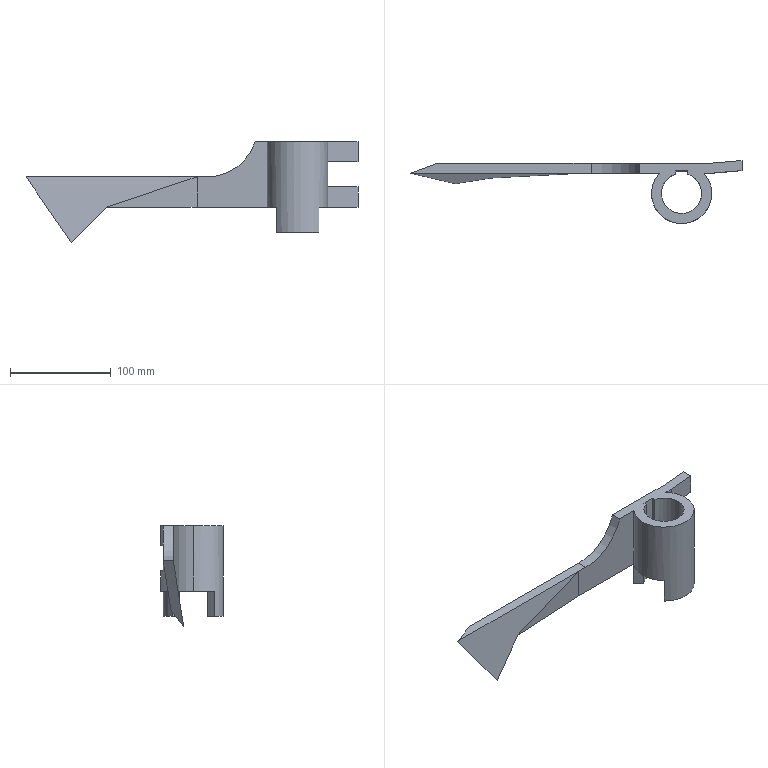Part | SolidWorks | features ICE 17, Extrusion 1, Rib 1 | 1 solid | 39 faces | box 330 x 62.625 x 100 mm | volume 226101 mm3 | plane 31 | cylinder 8 | commonest cylinder face diameters 60 x4 40 x3 100 x1
STEP:
#1=CARTESIAN_POINT('',(-20.,-20.,10.));
#2=VERTEX_POINT('',#1);
#3=CARTESIAN_POINT('',(20.,-20.,10.));
#4=VERTEX_POINT('',#3);
#5=CARTESIAN_POINT('',(0.,-20.,10.));
#6=DIRECTION('',(0.,0.,1.));
#7=DIRECTION('',(1.,0.,0.));
#8=AXIS2_PLACEMENT_3D('',#5,#6,#7);
#9=CIRCLE('',#8,20.);
#10=EDGE_CURVE('',#2,#4,#9,.T.);
#11=ORIENTED_EDGE('',*,*,#10,.T.);
#12=CARTESIAN_POINT('',(20.,-20.,-55.));
#13=VERTEX_POINT('',#12);
#14=CARTESIAN_POINT('',(20.,-20.,80.));
#15=DIRECTION('',(0.,0.,-1.));
#16=VECTOR('',#15,1000.);
#17=LINE('',#14,#16);
#18=EDGE_CURVE('',#4,#13,#17,.T.);
#19=ORIENTED_EDGE('',*,*,#18,.T.);
#20=CARTESIAN_POINT('',(14.142,-34.142,-55.));
#21=VERTEX_POINT('',#20);
#22=CARTESIAN_POINT('',(0.,-20.,-55.));
#23=DIRECTION('',(0.,0.,1.));
#24=DIRECTION('',(-1.,0.,0.));
#25=AXIS2_PLACEMENT_3D('',#22,#23,#24);
#26=CIRCLE('',#25,20.);
#27=EDGE_CURVE('',#21,#13,#26,.T.);
#28=ORIENTED_EDGE('',*,*,#27,.F.);
#29=CARTESIAN_POINT('',(14.142,-34.142,-80.));
#30=VERTEX_POINT('',#29);
#31=CARTESIAN_POINT('',(14.142,-34.142,-55.));
#32=DIRECTION('',(0.,0.,-1.));
#33=VECTOR('',#32,1000.);
#34=LINE('',#31,#33);
#35=EDGE_CURVE('',#21,#30,#34,.T.);
#36=ORIENTED_EDGE('',*,*,#35,.T.);
#37=CARTESIAN_POINT('',(-14.142,-34.142,-80.));
#38=VERTEX_POINT('',#37);
#39=CARTESIAN_POINT('',(0.,-20.,-80.));
#40=DIRECTION('',(0.,0.,1.));
#41=DIRECTION('',(1.,0.,0.));
#42=AXIS2_PLACEMENT_3D('',#39,#40,#41);
#43=CIRCLE('',#42,20.);
#44=EDGE_CURVE('',#38,#30,#43,.T.);
#45=ORIENTED_EDGE('',*,*,#44,.F.);
#46=CARTESIAN_POINT('',(-14.142,-34.142,-55.));
#47=VERTEX_POINT('',#46);
#48=CARTESIAN_POINT('',(-14.142,-34.142,-55.));
#49=DIRECTION('',(0.,0.,-1.));
#50=VECTOR('',#49,1000.);
#51=LINE('',#48,#50);
#52=EDGE_CURVE('',#47,#38,#51,.T.);
#53=ORIENTED_EDGE('',*,*,#52,.F.);
#54=CARTESIAN_POINT('',(-20.,-20.,-55.));
#55=VERTEX_POINT('',#54);
#56=CARTESIAN_POINT('',(0.,-20.,-55.));
#57=DIRECTION('',(0.,0.,1.));
#58=DIRECTION('',(-1.,0.,0.));
#59=AXIS2_PLACEMENT_3D('',#56,#57,#58);
#60=CIRCLE('',#59,20.);
#61=EDGE_CURVE('',#55,#47,#60,.T.);
#62=ORIENTED_EDGE('',*,*,#61,.F.);
#63=CARTESIAN_POINT('',(-20.,-20.,80.));
#64=DIRECTION('',(0.,0.,-1.));
#65=VECTOR('',#64,1000.);
#66=LINE('',#63,#65);
#67=EDGE_CURVE('',#2,#55,#66,.T.);
#68=ORIENTED_EDGE('',*,*,#67,.F.);
#69=EDGE_LOOP('',(#11,#19,#28,#36,#45,#53,#62,#68));
#70=FACE_OUTER_BOUND('',#69,.T.);
#71=CARTESIAN_POINT('',(0.,-20.,80.));
#72=DIRECTION('',(0.,0.,-1.));
#73=DIRECTION('',(-1.,0.,0.));
#74=AXIS2_PLACEMENT_3D('',#71,#72,#73);
#75=CYLINDRICAL_SURFACE('',#74,20.);
#76=ADVANCED_FACE('',(#70),#75,.F.);
#77=CARTESIAN_POINT('',(-6.,-0.9212,10.));
#78=VERTEX_POINT('',#77);
#79=CARTESIAN_POINT('',(0.,-20.,10.));
#80=DIRECTION('',(0.,0.,1.));
#81=DIRECTION('',(1.,0.,0.));
#82=AXIS2_PLACEMENT_3D('',#79,#80,#81);
#83=CIRCLE('',#82,20.);
#84=EDGE_CURVE('',#78,#2,#83,.T.);
#85=ORIENTED_EDGE('',*,*,#84,.T.);
#86=ORIENTED_EDGE('',*,*,#67,.T.);
#87=CARTESIAN_POINT('',(-14.142,-5.858,-55.));
#88=VERTEX_POINT('',#87);
#89=CARTESIAN_POINT('',(0.,-20.,-55.));
#90=DIRECTION('',(0.,0.,1.));
#91=DIRECTION('',(-1.,0.,0.));
#92=AXIS2_PLACEMENT_3D('',#89,#90,#91);
#93=CIRCLE('',#92,20.);
#94=EDGE_CURVE('',#88,#55,#93,.T.);
#95=ORIENTED_EDGE('',*,*,#94,.F.);
#96=CARTESIAN_POINT('',(-14.142,-5.858,-80.));
#97=VERTEX_POINT('',#96);
#98=CARTESIAN_POINT('',(-14.142,-5.858,-55.));
#99=DIRECTION('',(0.,0.,-1.));
#100=VECTOR('',#99,1000.);
#101=LINE('',#98,#100);
#102=EDGE_CURVE('',#88,#97,#101,.T.);
#103=ORIENTED_EDGE('',*,*,#102,.T.);
#104=CARTESIAN_POINT('',(-6.,-0.9212,-80.));
#105=VERTEX_POINT('',#104);
#106=CARTESIAN_POINT('',(0.,-20.,-80.));
#107=DIRECTION('',(0.,0.,1.));
#108=DIRECTION('',(1.,0.,0.));
#109=AXIS2_PLACEMENT_3D('',#106,#107,#108);
#110=CIRCLE('',#109,20.);
#111=EDGE_CURVE('',#105,#97,#110,.T.);
#112=ORIENTED_EDGE('',*,*,#111,.F.);
#113=CARTESIAN_POINT('',(-6.,-0.9212,80.));
#114=DIRECTION('',(0.,0.,-1.));
#115=VECTOR('',#114,1000.);
#116=LINE('',#113,#115);
#117=EDGE_CURVE('',#78,#105,#116,.T.);
#118=ORIENTED_EDGE('',*,*,#117,.F.);
#119=EDGE_LOOP('',(#85,#86,#95,#103,#112,#118));
#120=FACE_OUTER_BOUND('',#119,.T.);
#121=CARTESIAN_POINT('',(0.,-20.,80.));
#122=DIRECTION('',(0.,0.,-1.));
#123=DIRECTION('',(-1.,0.,0.));
#124=AXIS2_PLACEMENT_3D('',#121,#122,#123);
#125=CYLINDRICAL_SURFACE('',#124,20.);
#126=ADVANCED_FACE('',(#120),#125,.F.);
#127=CARTESIAN_POINT('',(30.,-20.,10.));
#128=VERTEX_POINT('',#127);
#129=CARTESIAN_POINT('',(22.361,0.,10.));
#130=VERTEX_POINT('',#129);
#131=CARTESIAN_POINT('',(0.,-20.,10.));
#132=DIRECTION('',(0.,0.,1.));
#133=DIRECTION('',(1.,0.,0.));
#134=AXIS2_PLACEMENT_3D('',#131,#132,#133);
#135=CIRCLE('',#134,30.);
#136=EDGE_CURVE('',#128,#130,#135,.T.);
#137=ORIENTED_EDGE('',*,*,#136,.F.);
#138=CARTESIAN_POINT('',(30.,-20.,-55.));
#139=VERTEX_POINT('',#138);
#140=CARTESIAN_POINT('',(30.,-20.,80.));
#141=DIRECTION('',(0.,0.,-1.));
#142=VECTOR('',#141,1000.);
#143=LINE('',#140,#142);
#144=EDGE_CURVE('',#128,#139,#143,.T.);
#145=ORIENTED_EDGE('',*,*,#144,.T.);
#146=CARTESIAN_POINT('',(22.361,0.,-55.));
#147=VERTEX_POINT('',#146);
#148=CARTESIAN_POINT('',(0.,-20.,-55.));
#149=DIRECTION('',(0.,0.,-1.));
#150=DIRECTION('',(-1.,0.,0.));
#151=AXIS2_PLACEMENT_3D('',#148,#149,#150);
#152=CIRCLE('',#151,30.);
#153=EDGE_CURVE('',#147,#139,#152,.T.);
#154=ORIENTED_EDGE('',*,*,#153,.F.);
#155=CARTESIAN_POINT('',(22.361,0.,-35.));
#156=VERTEX_POINT('',#155);
#157=CARTESIAN_POINT('',(22.361,0.,80.));
#158=DIRECTION('',(0.,0.,-1.));
#159=VECTOR('',#158,1000.);
#160=LINE('',#157,#159);
#161=EDGE_CURVE('',#156,#147,#160,.T.);
#162=ORIENTED_EDGE('',*,*,#161,.F.);
#163=CARTESIAN_POINT('',(0.,10.,-35.));
#164=VERTEX_POINT('',#163);
#165=CARTESIAN_POINT('',(0.,-20.,-35.));
#166=DIRECTION('',(0.,0.,1.));
#167=DIRECTION('',(-1.,0.,0.));
#168=AXIS2_PLACEMENT_3D('',#165,#166,#167);
#169=CIRCLE('',#168,30.);
#170=EDGE_CURVE('',#156,#164,#169,.T.);
#171=ORIENTED_EDGE('',*,*,#170,.T.);
#172=CARTESIAN_POINT('',(0.,10.,-10.));
#173=VERTEX_POINT('',#172);
#174=CARTESIAN_POINT('',(0.,10.,-10.));
#175=DIRECTION('',(0.,0.,-1.));
#176=VECTOR('',#175,1000.);
#177=LINE('',#174,#176);
#178=EDGE_CURVE('',#173,#164,#177,.T.);
#179=ORIENTED_EDGE('',*,*,#178,.F.);
#180=CARTESIAN_POINT('',(22.361,0.,-10.));
#181=VERTEX_POINT('',#180);
#182=CARTESIAN_POINT('',(0.,-20.,-10.));
#183=DIRECTION('',(0.,0.,-1.));
#184=DIRECTION('',(-1.,0.,0.));
#185=AXIS2_PLACEMENT_3D('',#182,#183,#184);
#186=CIRCLE('',#185,30.);
#187=EDGE_CURVE('',#173,#181,#186,.T.);
#188=ORIENTED_EDGE('',*,*,#187,.T.);
#189=CARTESIAN_POINT('',(22.361,0.,80.));
#190=DIRECTION('',(0.,0.,-1.));
#191=VECTOR('',#190,1000.);
#192=LINE('',#189,#191);
#193=EDGE_CURVE('',#130,#181,#192,.T.);
#194=ORIENTED_EDGE('',*,*,#193,.F.);
#195=EDGE_LOOP('',(#137,#145,#154,#162,#171,#179,#188,#194));
#196=FACE_OUTER_BOUND('',#195,.T.);
#197=CARTESIAN_POINT('',(0.,-20.,80.));
#198=DIRECTION('',(0.,0.,-1.));
#199=DIRECTION('',(-1.,0.,0.));
#200=AXIS2_PLACEMENT_3D('',#197,#198,#199);
#201=CYLINDRICAL_SURFACE('',#200,30.);
#202=ADVANCED_FACE('',(#196),#201,.T.);
#203=ORIENTED_EDGE('',*,*,#144,.F.);
#204=CARTESIAN_POINT('',(-30.,-20.,10.));
#205=VERTEX_POINT('',#204);
#206=CARTESIAN_POINT('',(0.,-20.,10.));
#207=DIRECTION('',(0.,0.,1.));
#208=DIRECTION('',(1.,0.,0.));
#209=AXIS2_PLACEMENT_3D('',#206,#207,#208);
#210=CIRCLE('',#209,30.);
#211=EDGE_CURVE('',#205,#128,#210,.T.);
#212=ORIENTED_EDGE('',*,*,#211,.F.);
#213=CARTESIAN_POINT('',(-30.,-20.,-55.));
#214=VERTEX_POINT('',#213);
#215=CARTESIAN_POINT('',(-30.,-20.,80.));
#216=DIRECTION('',(0.,0.,-1.));
#217=VECTOR('',#216,1000.);
#218=LINE('',#215,#217);
#219=EDGE_CURVE('',#205,#214,#218,.T.);
#220=ORIENTED_EDGE('',*,*,#219,.T.);
#221=CARTESIAN_POINT('',(-21.213,-41.213,-55.));
#222=VERTEX_POINT('',#221);
#223=CARTESIAN_POINT('',(0.,-20.,-55.));
#224=DIRECTION('',(0.,0.,-1.));
#225=DIRECTION('',(-1.,0.,0.));
#226=AXIS2_PLACEMENT_3D('',#223,#224,#225);
#227=CIRCLE('',#226,30.);
#228=EDGE_CURVE('',#222,#214,#227,.T.);
#229=ORIENTED_EDGE('',*,*,#228,.F.);
#230=CARTESIAN_POINT('',(-21.213,-41.213,-80.));
#231=VERTEX_POINT('',#230);
#232=CARTESIAN_POINT('',(-21.213,-41.213,-55.));
#233=DIRECTION('',(0.,0.,-1.));
#234=VECTOR('',#233,1000.);
#235=LINE('',#232,#234);
#236=EDGE_CURVE('',#222,#231,#235,.T.);
#237=ORIENTED_EDGE('',*,*,#236,.T.);
#238=CARTESIAN_POINT('',(21.213,-41.213,-80.));
#239=VERTEX_POINT('',#238);
#240=CARTESIAN_POINT('',(0.,-20.,-80.));
#241=DIRECTION('',(0.,0.,1.));
#242=DIRECTION('',(1.,0.,0.));
#243=AXIS2_PLACEMENT_3D('',#240,#241,#242);
#244=CIRCLE('',#243,30.);
#245=EDGE_CURVE('',#231,#239,#244,.T.);
#246=ORIENTED_EDGE('',*,*,#245,.T.);
#247=CARTESIAN_POINT('',(21.213,-41.213,-55.));
#248=VERTEX_POINT('',#247);
#249=CARTESIAN_POINT('',(21.213,-41.213,-55.));
#250=DIRECTION('',(0.,0.,-1.));
#251=VECTOR('',#250,1000.);
#252=LINE('',#249,#251);
#253=EDGE_CURVE('',#248,#239,#252,.T.);
#254=ORIENTED_EDGE('',*,*,#253,.F.);
#255=CARTESIAN_POINT('',(0.,-20.,-55.));
#256=DIRECTION('',(0.,0.,-1.));
#257=DIRECTION('',(-1.,0.,0.));
#258=AXIS2_PLACEMENT_3D('',#255,#256,#257);
#259=CIRCLE('',#258,30.);
#260=EDGE_CURVE('',#139,#248,#259,.T.);
#261=ORIENTED_EDGE('',*,*,#260,.F.);
#262=EDGE_LOOP('',(#203,#212,#220,#229,#237,#246,#254,#261));
#263=FACE_OUTER_BOUND('',#262,.T.);
#264=CARTESIAN_POINT('',(0.,-20.,80.));
#265=DIRECTION('',(0.,0.,-1.));
#266=DIRECTION('',(-1.,0.,0.));
#267=AXIS2_PLACEMENT_3D('',#264,#265,#266);
#268=CYLINDRICAL_SURFACE('',#267,30.);
#269=ADVANCED_FACE('',(#263),#268,.T.);
#270=ORIENTED_EDGE('',*,*,#219,.F.);
#271=CARTESIAN_POINT('',(-22.361,0.,10.));
#272=VERTEX_POINT('',#271);
#273=CARTESIAN_POINT('',(0.,-20.,10.));
#274=DIRECTION('',(0.,0.,1.));
#275=DIRECTION('',(1.,0.,0.));
#276=AXIS2_PLACEMENT_3D('',#273,#274,#275);
#277=CIRCLE('',#276,30.);
#278=EDGE_CURVE('',#272,#205,#277,.T.);
#279=ORIENTED_EDGE('',*,*,#278,.F.);
#280=CARTESIAN_POINT('',(-22.361,0.,-55.));
#281=VERTEX_POINT('',#280);
#282=CARTESIAN_POINT('',(-22.361,0.,80.));
#283=DIRECTION('',(0.,0.,1.));
#284=VECTOR('',#283,1000.);
#285=LINE('',#282,#284);
#286=EDGE_CURVE('',#281,#272,#285,.T.);
#287=ORIENTED_EDGE('',*,*,#286,.F.);
#288=CARTESIAN_POINT('',(0.,-20.,-55.));
#289=DIRECTION('',(0.,0.,-1.));
#290=DIRECTION('',(-1.,0.,0.));
#291=AXIS2_PLACEMENT_3D('',#288,#289,#290);
#292=CIRCLE('',#291,30.);
#293=EDGE_CURVE('',#214,#281,#292,.T.);
#294=ORIENTED_EDGE('',*,*,#293,.F.);
#295=EDGE_LOOP('',(#270,#279,#287,#294));
#296=FACE_OUTER_BOUND('',#295,.T.);
#297=CARTESIAN_POINT('',(0.,-20.,80.));
#298=DIRECTION('',(0.,0.,-1.));
#299=DIRECTION('',(-1.,0.,0.));
#300=AXIS2_PLACEMENT_3D('',#297,#298,#299);
#301=CYLINDRICAL_SURFACE('',#300,30.);
#302=ADVANCED_FACE('',(#296),#301,.T.);
#303=ORIENTED_EDGE('',*,*,#286,.T.);
#304=CARTESIAN_POINT('',(-42.303,0.,10.));
#305=VERTEX_POINT('',#304);
#306=CARTESIAN_POINT('',(-40.,0.,10.));
#307=DIRECTION('',(1.,0.,0.));
#308=VECTOR('',#307,1000.);
#309=LINE('',#306,#308);
#310=EDGE_CURVE('',#305,#272,#309,.T.);
#311=ORIENTED_EDGE('',*,*,#310,.F.);
#312=CARTESIAN_POINT('',(-90.,0.,-25.));
#313=VERTEX_POINT('',#312);
#314=CARTESIAN_POINT('',(-90.,0.,25.));
#315=DIRECTION('',(0.,-1.,0.));
#316=DIRECTION('',(0.,0.,1.));
#317=AXIS2_PLACEMENT_3D('',#314,#315,#316);
#318=CIRCLE('',#317,50.);
#319=EDGE_CURVE('',#313,#305,#318,.T.);
#320=ORIENTED_EDGE('',*,*,#319,.F.);
#321=CARTESIAN_POINT('',(-100.,0.,-25.));
#322=VERTEX_POINT('',#321);
#323=CARTESIAN_POINT('',(0.,0.,-25.));
#324=DIRECTION('',(-1.,0.,0.));
#325=VECTOR('',#324,1000.);
#326=LINE('',#323,#325);
#327=EDGE_CURVE('',#313,#322,#326,.T.);
#328=ORIENTED_EDGE('',*,*,#327,.T.);
#329=CARTESIAN_POINT('',(-100.,0.,-55.));
#330=VERTEX_POINT('',#329);
#331=CARTESIAN_POINT('',(-100.,0.,-55.));
#332=DIRECTION('',(0.,0.,1.));
#333=VECTOR('',#332,1000.);
#334=LINE('',#331,#333);
#335=EDGE_CURVE('',#330,#322,#334,.T.);
#336=ORIENTED_EDGE('',*,*,#335,.F.);
#337=CARTESIAN_POINT('',(30.,0.,-55.));
#338=DIRECTION('',(-1.,0.,0.));
#339=VECTOR('',#338,1000.);
#340=LINE('',#337,#339);
#341=EDGE_CURVE('',#281,#330,#340,.T.);
#342=ORIENTED_EDGE('',*,*,#341,.F.);
#343=EDGE_LOOP('',(#303,#311,#320,#328,#336,#342));
#344=FACE_OUTER_BOUND('',#343,.T.);
#345=CARTESIAN_POINT('',(0.,0.,0.));
#346=DIRECTION('',(0.,-1.,0.));
#347=DIRECTION('',(0.,0.,-1.));
#348=AXIS2_PLACEMENT_3D('',#345,#346,#347);
#349=PLANE('',#348);
#350=ADVANCED_FACE('',(#344),#349,.T.);
#351=CARTESIAN_POINT('',(-90.,10.,-25.));
#352=VERTEX_POINT('',#351);
#353=CARTESIAN_POINT('',(-100.,10.,-25.));
#354=VERTEX_POINT('',#353);
#355=CARTESIAN_POINT('',(0.,10.,-25.));
#356=DIRECTION('',(-1.,0.,0.));
#357=VECTOR('',#356,1000.);
#358=LINE('',#355,#357);
#359=EDGE_CURVE('',#352,#354,#358,.T.);
#360=ORIENTED_EDGE('',*,*,#359,.F.);
#361=CARTESIAN_POINT('',(-42.303,10.,10.));
#362=VERTEX_POINT('',#361);
#363=CARTESIAN_POINT('',(-90.,10.,25.));
#364=DIRECTION('',(0.,-1.,0.));
#365=DIRECTION('',(0.,0.,1.));
#366=AXIS2_PLACEMENT_3D('',#363,#364,#365);
#367=CIRCLE('',#366,50.);
#368=EDGE_CURVE('',#352,#362,#367,.T.);
#369=ORIENTED_EDGE('',*,*,#368,.T.);
#370=CARTESIAN_POINT('',(30.,10.,10.));
#371=VERTEX_POINT('',#370);
#372=CARTESIAN_POINT('',(30.,10.,10.));
#373=DIRECTION('',(1.,0.,0.));
#374=VECTOR('',#373,1000.);
#375=LINE('',#372,#374);
#376=EDGE_CURVE('',#362,#371,#375,.T.);
#377=ORIENTED_EDGE('',*,*,#376,.T.);
#378=CARTESIAN_POINT('',(30.,10.,-10.));
#379=VERTEX_POINT('',#378);
#380=CARTESIAN_POINT('',(30.,10.,-10.));
#381=DIRECTION('',(0.,0.,-1.));
#382=VECTOR('',#381,1000.);
#383=LINE('',#380,#382);
#384=EDGE_CURVE('',#371,#379,#383,.T.);
#385=ORIENTED_EDGE('',*,*,#384,.T.);
#386=CARTESIAN_POINT('',(0.,10.,-10.));
#387=DIRECTION('',(-1.,0.,0.));
#388=VECTOR('',#387,1000.);
#389=LINE('',#386,#388);
#390=EDGE_CURVE('',#379,#173,#389,.T.);
#391=ORIENTED_EDGE('',*,*,#390,.T.);
#392=ORIENTED_EDGE('',*,*,#178,.T.);
#393=CARTESIAN_POINT('',(30.,10.,-35.));
#394=VERTEX_POINT('',#393);
#395=CARTESIAN_POINT('',(0.,10.,-35.));
#396=DIRECTION('',(1.,0.,0.));
#397=VECTOR('',#396,1000.);
#398=LINE('',#395,#397);
#399=EDGE_CURVE('',#164,#394,#398,.T.);
#400=ORIENTED_EDGE('',*,*,#399,.T.);
#401=CARTESIAN_POINT('',(30.,10.,-55.));
#402=VERTEX_POINT('',#401);
#403=CARTESIAN_POINT('',(30.,10.,-35.));
#404=DIRECTION('',(0.,0.,-1.));
#405=VECTOR('',#404,1000.);
#406=LINE('',#403,#405);
#407=EDGE_CURVE('',#394,#402,#406,.T.);
#408=ORIENTED_EDGE('',*,*,#407,.T.);
#409=CARTESIAN_POINT('',(0.,10.,-55.));
#410=VERTEX_POINT('',#409);
#411=CARTESIAN_POINT('',(30.,10.,-55.));
#412=DIRECTION('',(-1.,0.,0.));
#413=VECTOR('',#412,1000.);
#414=LINE('',#411,#413);
#415=EDGE_CURVE('',#402,#410,#414,.T.);
#416=ORIENTED_EDGE('',*,*,#415,.T.);
#417=CARTESIAN_POINT('',(-100.,10.,-55.));
#418=VERTEX_POINT('',#417);
#419=CARTESIAN_POINT('',(30.,10.,-55.));
#420=DIRECTION('',(-1.,0.,0.));
#421=VECTOR('',#420,1000.);
#422=LINE('',#419,#421);
#423=EDGE_CURVE('',#410,#418,#422,.T.);
#424=ORIENTED_EDGE('',*,*,#423,.T.);
#425=CARTESIAN_POINT('',(-100.,10.,-55.));
#426=DIRECTION('',(0.,0.,1.));
#427=VECTOR('',#426,1000.);
#428=LINE('',#425,#427);
#429=EDGE_CURVE('',#418,#354,#428,.T.);
#430=ORIENTED_EDGE('',*,*,#429,.T.);
#431=EDGE_LOOP('',(#360,#369,#377,#385,#391,#392,#400,#408,#416,#424,#430));
#432=FACE_OUTER_BOUND('',#431,.T.);
#433=CARTESIAN_POINT('',(0.,10.,0.));
#434=DIRECTION('',(0.,-1.,0.));
#435=DIRECTION('',(0.,0.,-1.));
#436=AXIS2_PLACEMENT_3D('',#433,#434,#435);
#437=PLANE('',#436);
#438=ADVANCED_FACE('',(#432),#437,.F.);
#439=ORIENTED_EDGE('',*,*,#18,.F.);
#440=CARTESIAN_POINT('',(6.,-0.9212,10.));
#441=VERTEX_POINT('',#440);
#442=CARTESIAN_POINT('',(0.,-20.,10.));
#443=DIRECTION('',(0.,0.,1.));
#444=DIRECTION('',(1.,0.,0.));
#445=AXIS2_PLACEMENT_3D('',#442,#443,#444);
#446=CIRCLE('',#445,20.);
#447=EDGE_CURVE('',#4,#441,#446,.T.);
#448=ORIENTED_EDGE('',*,*,#447,.T.);
#449=CARTESIAN_POINT('',(6.,-0.9212,-80.));
#450=VERTEX_POINT('',#449);
#451=CARTESIAN_POINT('',(6.,-0.9212,80.));
#452=DIRECTION('',(0.,0.,1.));
#453=VECTOR('',#452,1000.);
#454=LINE('',#451,#453);
#455=EDGE_CURVE('',#450,#441,#454,.T.);
#456=ORIENTED_EDGE('',*,*,#455,.F.);
#457=CARTESIAN_POINT('',(14.142,-5.858,-80.));
#458=VERTEX_POINT('',#457);
#459=CARTESIAN_POINT('',(0.,-20.,-80.));
#460=DIRECTION('',(0.,0.,1.));
#461=DIRECTION('',(1.,0.,0.));
#462=AXIS2_PLACEMENT_3D('',#459,#460,#461);
#463=CIRCLE('',#462,20.);
#464=EDGE_CURVE('',#458,#450,#463,.T.);
#465=ORIENTED_EDGE('',*,*,#464,.F.);
#466=CARTESIAN_POINT('',(14.142,-5.858,-55.));
#467=VERTEX_POINT('',#466);
#468=CARTESIAN_POINT('',(14.142,-5.858,-55.));
#469=DIRECTION('',(0.,0.,-1.));
#470=VECTOR('',#469,1000.);
#471=LINE('',#468,#470);
#472=EDGE_CURVE('',#467,#458,#471,.T.);
#473=ORIENTED_EDGE('',*,*,#472,.F.);
#474=CARTESIAN_POINT('',(0.,-20.,-55.));
#475=DIRECTION('',(0.,0.,1.));
#476=DIRECTION('',(-1.,0.,0.));
#477=AXIS2_PLACEMENT_3D('',#474,#475,#476);
#478=CIRCLE('',#477,20.);
#479=EDGE_CURVE('',#13,#467,#478,.T.);
#480=ORIENTED_EDGE('',*,*,#479,.F.);
#481=EDGE_LOOP('',(#439,#448,#456,#465,#473,#480));
#482=FACE_OUTER_BOUND('',#481,.T.);
#483=CARTESIAN_POINT('',(0.,-20.,80.));
#484=DIRECTION('',(0.,0.,-1.));
#485=DIRECTION('',(-1.,0.,0.));
#486=AXIS2_PLACEMENT_3D('',#483,#484,#485);
#487=CYLINDRICAL_SURFACE('',#486,20.);
#488=ADVANCED_FACE('',(#482),#487,.F.);
#489=CARTESIAN_POINT('',(-270.,0.,-25.));
#490=VERTEX_POINT('',#489);
#491=CARTESIAN_POINT('',(-225.,-10.295,-90.));
#492=VERTEX_POINT('',#491);
#493=CARTESIAN_POINT('',(-239.337,-7.015,-69.291));
#494=DIRECTION('',(0.5644,-0.1291,-0.8153));
#495=VECTOR('',#494,1000.);
#496=LINE('',#493,#495);
#497=EDGE_CURVE('',#490,#492,#496,.T.);
#498=ORIENTED_EDGE('',*,*,#497,.F.);
#499=CARTESIAN_POINT('',(-242.732,10.,-25.));
#500=VERTEX_POINT('',#499);
#501=CARTESIAN_POINT('',(-270.,0.,-25.));
#502=DIRECTION('',(0.9389,0.3443,0.));
#503=VECTOR('',#502,1000.);
#504=LINE('',#501,#503);
#505=EDGE_CURVE('',#490,#500,#504,.T.);
#506=ORIENTED_EDGE('',*,*,#505,.T.);
#507=CARTESIAN_POINT('',(-208.887,2.257,-73.887));
#508=VERTEX_POINT('',#507);
#509=CARTESIAN_POINT('',(-220.757,4.972,-56.743));
#510=DIRECTION('',(0.5644,-0.1291,-0.8153));
#511=VECTOR('',#510,1000.);
#512=LINE('',#509,#511);
#513=EDGE_CURVE('',#500,#508,#512,.T.);
#514=ORIENTED_EDGE('',*,*,#513,.T.);
#515=CARTESIAN_POINT('',(-242.884,-24.227,-107.884));
#516=DIRECTION('',(-0.6194,-0.4825,-0.6194));
#517=VECTOR('',#516,1000.);
#518=LINE('',#515,#517);
#519=EDGE_CURVE('',#508,#492,#518,.T.);
#520=ORIENTED_EDGE('',*,*,#519,.T.);
#521=EDGE_LOOP('',(#498,#506,#514,#520));
#522=FACE_OUTER_BOUND('',#521,.T.);
#523=CARTESIAN_POINT('',(-30.735,83.808,-34.552));
#524=DIRECTION('',(-0.3211,0.8756,-0.361));
#525=DIRECTION('',(0.,0.3812,0.9245));
#526=AXIS2_PLACEMENT_3D('',#523,#524,#525);
#527=PLANE('',#526);
#528=ADVANCED_FACE('',(#522),#527,.T.);
#529=ORIENTED_EDGE('',*,*,#513,.F.);
#530=CARTESIAN_POINT('',(-270.,10.,-25.));
#531=DIRECTION('',(1.,0.,0.));
#532=VECTOR('',#531,1000.);
#533=LINE('',#530,#532);
#534=EDGE_CURVE('',#500,#354,#533,.T.);
#535=ORIENTED_EDGE('',*,*,#534,.T.);
#536=CARTESIAN_POINT('',(-190.,5.248,-55.));
#537=VERTEX_POINT('',#536);
#538=CARTESIAN_POINT('',(-272.556,0.8899,-82.519));
#539=DIRECTION('',(-0.9475,-0.05002,-0.3158));
#540=VECTOR('',#539,1000.);
#541=LINE('',#538,#540);
#542=EDGE_CURVE('',#354,#537,#541,.T.);
#543=ORIENTED_EDGE('',*,*,#542,.T.);
#544=CARTESIAN_POINT('',(-247.221,-3.814,-112.221));
#545=DIRECTION('',(-0.7027,-0.1113,-0.7027));
#546=VECTOR('',#545,1000.);
#547=LINE('',#544,#546);
#548=EDGE_CURVE('',#537,#508,#547,.T.);
#549=ORIENTED_EDGE('',*,*,#548,.T.);
#550=EDGE_LOOP('',(#529,#535,#543,#549));
#551=FACE_OUTER_BOUND('',#550,.T.);
#552=CARTESIAN_POINT('',(-270.,-0.295,-90.));
#553=DIRECTION('',(0.,-0.9877,0.1564));
#554=DIRECTION('',(0.,-0.1564,-0.9877));
#555=AXIS2_PLACEMENT_3D('',#552,#553,#554);
#556=PLANE('',#555);
#557=ADVANCED_FACE('',(#551),#556,.F.);
#558=ORIENTED_EDGE('',*,*,#519,.F.);
#559=ORIENTED_EDGE('',*,*,#548,.F.);
#560=CARTESIAN_POINT('',(-190.,-4.752,-55.));
#561=VERTEX_POINT('',#560);
#562=CARTESIAN_POINT('',(-190.,-160.,-55.));
#563=DIRECTION('',(0.,1.,0.));
#564=VECTOR('',#563,1000.);
#565=LINE('',#562,#564);
#566=EDGE_CURVE('',#561,#537,#565,.T.);
#567=ORIENTED_EDGE('',*,*,#566,.F.);
#568=CARTESIAN_POINT('',(-247.221,-13.814,-112.221));
#569=DIRECTION('',(0.7027,0.1113,0.7027));
#570=VECTOR('',#569,1000.);
#571=LINE('',#568,#570);
#572=EDGE_CURVE('',#492,#561,#571,.T.);
#573=ORIENTED_EDGE('',*,*,#572,.F.);
#574=EDGE_LOOP('',(#558,#559,#567,#573));
#575=FACE_OUTER_BOUND('',#574,.T.);
#576=CARTESIAN_POINT('',(-190.,-160.,-55.));
#577=DIRECTION('',(-0.7071,0.,0.7071));
#578=DIRECTION('',(0.7071,0.,0.7071));
#579=AXIS2_PLACEMENT_3D('',#576,#577,#578);
#580=PLANE('',#579);
#581=ADVANCED_FACE('',(#575),#580,.F.);
#582=ORIENTED_EDGE('',*,*,#245,.F.);
#583=CARTESIAN_POINT('',(-14.142,-34.142,-80.));
#584=DIRECTION('',(-0.7071,-0.7071,0.));
#585=VECTOR('',#584,1000.);
#586=LINE('',#583,#585);
#587=EDGE_CURVE('',#38,#231,#586,.T.);
#588=ORIENTED_EDGE('',*,*,#587,.F.);
#589=ORIENTED_EDGE('',*,*,#44,.T.);
#590=CARTESIAN_POINT('',(21.213,-41.213,-80.));
#591=DIRECTION('',(-0.7071,0.7071,0.));
#592=VECTOR('',#591,1000.);
#593=LINE('',#590,#592);
#594=EDGE_CURVE('',#239,#30,#593,.T.);
#595=ORIENTED_EDGE('',*,*,#594,.F.);
#596=EDGE_LOOP('',(#582,#588,#589,#595));
#597=FACE_OUTER_BOUND('',#596,.T.);
#598=CARTESIAN_POINT('',(0.,-20.,-80.));
#599=DIRECTION('',(0.,0.,1.));
#600=DIRECTION('',(1.,0.,0.));
#601=AXIS2_PLACEMENT_3D('',#598,#599,#600);
#602=PLANE('',#601);
#603=ADVANCED_FACE('',(#597),#602,.F.);
#604=CARTESIAN_POINT('',(21.213,1.213,-80.));
#605=VERTEX_POINT('',#604);
#606=CARTESIAN_POINT('',(-21.213,1.213,-80.));
#607=VERTEX_POINT('',#606);
#608=CARTESIAN_POINT('',(0.,-20.,-80.));
#609=DIRECTION('',(0.,0.,1.));
#610=DIRECTION('',(1.,0.,0.));
#611=AXIS2_PLACEMENT_3D('',#608,#609,#610);
#612=CIRCLE('',#611,30.);
#613=EDGE_CURVE('',#605,#607,#612,.T.);
#614=ORIENTED_EDGE('',*,*,#613,.T.);
#615=CARTESIAN_POINT('',(-21.213,1.213,-55.));
#616=VERTEX_POINT('',#615);
#617=CARTESIAN_POINT('',(-21.213,1.213,-55.));
#618=DIRECTION('',(0.,0.,-1.));
#619=VECTOR('',#618,1000.);
#620=LINE('',#617,#619);
#621=EDGE_CURVE('',#616,#607,#620,.T.);
#622=ORIENTED_EDGE('',*,*,#621,.F.);
#623=CARTESIAN_POINT('',(0.,-20.,-55.));
#624=DIRECTION('',(0.,0.,-1.));
#625=DIRECTION('',(1.,0.,0.));
#626=AXIS2_PLACEMENT_3D('',#623,#624,#625);
#627=CIRCLE('',#626,30.);
#628=EDGE_CURVE('',#616,#410,#627,.T.);
#629=ORIENTED_EDGE('',*,*,#628,.T.);
#630=CARTESIAN_POINT('',(21.213,1.213,-55.));
#631=VERTEX_POINT('',#630);
#632=CARTESIAN_POINT('',(0.,-20.,-55.));
#633=DIRECTION('',(0.,0.,-1.));
#634=DIRECTION('',(1.,0.,0.));
#635=AXIS2_PLACEMENT_3D('',#632,#633,#634);
#636=CIRCLE('',#635,30.);
#637=EDGE_CURVE('',#410,#631,#636,.T.);
#638=ORIENTED_EDGE('',*,*,#637,.T.);
#639=CARTESIAN_POINT('',(21.213,1.213,-55.));
#640=DIRECTION('',(0.,0.,-1.));
#641=VECTOR('',#640,1000.);
#642=LINE('',#639,#641);
#643=EDGE_CURVE('',#631,#605,#642,.T.);
#644=ORIENTED_EDGE('',*,*,#643,.T.);
#645=EDGE_LOOP('',(#614,#622,#629,#638,#644));
#646=FACE_OUTER_BOUND('',#645,.T.);
#647=CARTESIAN_POINT('',(0.,-20.,80.));
#648=DIRECTION('',(0.,0.,-1.));
#649=DIRECTION('',(-1.,0.,0.));
#650=AXIS2_PLACEMENT_3D('',#647,#648,#649);
#651=CYLINDRICAL_SURFACE('',#650,30.);
#652=ADVANCED_FACE('',(#646),#651,.T.);
#653=ORIENTED_EDGE('',*,*,#170,.F.);
#654=CARTESIAN_POINT('',(30.,0.,-35.));
#655=VERTEX_POINT('',#654);
#656=CARTESIAN_POINT('',(0.,0.,-35.));
#657=DIRECTION('',(1.,0.,0.));
#658=VECTOR('',#657,1000.);
#659=LINE('',#656,#658);
#660=EDGE_CURVE('',#156,#655,#659,.T.);
#661=ORIENTED_EDGE('',*,*,#660,.T.);
#662=CARTESIAN_POINT('',(60.,2.625,-35.));
#663=VERTEX_POINT('',#662);
#664=CARTESIAN_POINT('',(30.,0.,-35.));
#665=DIRECTION('',(0.9962,0.08716,0.));
#666=VECTOR('',#665,1000.);
#667=LINE('',#664,#666);
#668=EDGE_CURVE('',#655,#663,#667,.T.);
#669=ORIENTED_EDGE('',*,*,#668,.T.);
#670=CARTESIAN_POINT('',(60.,12.625,-35.));
#671=VERTEX_POINT('',#670);
#672=CARTESIAN_POINT('',(60.,2.625,-35.));
#673=DIRECTION('',(0.,1.,0.));
#674=VECTOR('',#673,1000.);
#675=LINE('',#672,#674);
#676=EDGE_CURVE('',#663,#671,#675,.T.);
#677=ORIENTED_EDGE('',*,*,#676,.T.);
#678=CARTESIAN_POINT('',(30.,10.,-35.));
#679=DIRECTION('',(-0.9962,-0.08716,0.));
#680=VECTOR('',#679,1000.);
#681=LINE('',#678,#680);
#682=EDGE_CURVE('',#671,#394,#681,.T.);
#683=ORIENTED_EDGE('',*,*,#682,.T.);
#684=ORIENTED_EDGE('',*,*,#399,.F.);
#685=EDGE_LOOP('',(#653,#661,#669,#677,#683,#684));
#686=FACE_OUTER_BOUND('',#685,.T.);
#687=CARTESIAN_POINT('',(0.,10.,-35.));
#688=DIRECTION('',(0.,0.,-1.));
#689=DIRECTION('',(-1.,0.,0.));
#690=AXIS2_PLACEMENT_3D('',#687,#688,#689);
#691=PLANE('',#690);
#692=ADVANCED_FACE('',(#686),#691,.F.);
#693=ORIENTED_EDGE('',*,*,#628,.F.);
#694=CARTESIAN_POINT('',(-21.213,1.213,-55.));
#695=DIRECTION('',(0.7071,-0.7071,0.));
#696=VECTOR('',#695,1000.);
#697=LINE('',#694,#696);
#698=EDGE_CURVE('',#616,#88,#697,.T.);
#699=ORIENTED_EDGE('',*,*,#698,.T.);
#700=ORIENTED_EDGE('',*,*,#94,.T.);
#701=ORIENTED_EDGE('',*,*,#61,.T.);
#702=CARTESIAN_POINT('',(-14.142,-34.142,-55.));
#703=DIRECTION('',(-0.7071,-0.7071,0.));
#704=VECTOR('',#703,1000.);
#705=LINE('',#702,#704);
#706=EDGE_CURVE('',#47,#222,#705,.T.);
#707=ORIENTED_EDGE('',*,*,#706,.T.);
#708=ORIENTED_EDGE('',*,*,#228,.T.);
#709=ORIENTED_EDGE('',*,*,#293,.T.);
#710=ORIENTED_EDGE('',*,*,#341,.T.);
#711=CARTESIAN_POINT('',(-100.,0.,-55.));
#712=DIRECTION('',(-0.9986,-0.05272,0.));
#713=VECTOR('',#712,1000.);
#714=LINE('',#711,#713);
#715=EDGE_CURVE('',#330,#561,#714,.T.);
#716=ORIENTED_EDGE('',*,*,#715,.T.);
#717=ORIENTED_EDGE('',*,*,#566,.T.);
#718=CARTESIAN_POINT('',(-190.,5.248,-55.));
#719=DIRECTION('',(0.9986,0.05272,0.));
#720=VECTOR('',#719,1000.);
#721=LINE('',#718,#720);
#722=EDGE_CURVE('',#537,#418,#721,.T.);
#723=ORIENTED_EDGE('',*,*,#722,.T.);
#724=ORIENTED_EDGE('',*,*,#423,.F.);
#725=EDGE_LOOP('',(#693,#699,#700,#701,#707,#708,#709,#710,#716,#717,#723,#724));
#726=FACE_OUTER_BOUND('',#725,.T.);
#727=CARTESIAN_POINT('',(30.,10.,-55.));
#728=DIRECTION('',(0.,0.,1.));
#729=DIRECTION('',(1.,0.,0.));
#730=AXIS2_PLACEMENT_3D('',#727,#728,#729);
#731=PLANE('',#730);
#732=ADVANCED_FACE('',(#726),#731,.F.);
#733=ORIENTED_EDGE('',*,*,#637,.F.);
#734=ORIENTED_EDGE('',*,*,#415,.F.);
#735=CARTESIAN_POINT('',(60.,12.625,-55.));
#736=VERTEX_POINT('',#735);
#737=CARTESIAN_POINT('',(30.,10.,-55.));
#738=DIRECTION('',(-0.9962,-0.08716,0.));
#739=VECTOR('',#738,1000.);
#740=LINE('',#737,#739);
#741=EDGE_CURVE('',#736,#402,#740,.T.);
#742=ORIENTED_EDGE('',*,*,#741,.F.);
#743=CARTESIAN_POINT('',(60.,2.625,-55.));
#744=VERTEX_POINT('',#743);
#745=CARTESIAN_POINT('',(60.,2.625,-55.));
#746=DIRECTION('',(0.,1.,0.));
#747=VECTOR('',#746,1000.);
#748=LINE('',#745,#747);
#749=EDGE_CURVE('',#744,#736,#748,.T.);
#750=ORIENTED_EDGE('',*,*,#749,.F.);
#751=CARTESIAN_POINT('',(30.,0.,-55.));
#752=VERTEX_POINT('',#751);
#753=CARTESIAN_POINT('',(30.,0.,-55.));
#754=DIRECTION('',(0.9962,0.08716,0.));
#755=VECTOR('',#754,1000.);
#756=LINE('',#753,#755);
#757=EDGE_CURVE('',#752,#744,#756,.T.);
#758=ORIENTED_EDGE('',*,*,#757,.F.);
#759=CARTESIAN_POINT('',(30.,0.,-55.));
#760=DIRECTION('',(-1.,0.,0.));
#761=VECTOR('',#760,1000.);
#762=LINE('',#759,#761);
#763=EDGE_CURVE('',#752,#147,#762,.T.);
#764=ORIENTED_EDGE('',*,*,#763,.T.);
#765=ORIENTED_EDGE('',*,*,#153,.T.);
#766=ORIENTED_EDGE('',*,*,#260,.T.);
#767=CARTESIAN_POINT('',(21.213,-41.213,-55.));
#768=DIRECTION('',(-0.7071,0.7071,0.));
#769=VECTOR('',#768,1000.);
#770=LINE('',#767,#769);
#771=EDGE_CURVE('',#248,#21,#770,.T.);
#772=ORIENTED_EDGE('',*,*,#771,.T.);
#773=ORIENTED_EDGE('',*,*,#27,.T.);
#774=ORIENTED_EDGE('',*,*,#479,.T.);
#775=CARTESIAN_POINT('',(14.142,-5.858,-55.));
#776=DIRECTION('',(0.7071,0.7071,0.));
#777=VECTOR('',#776,1000.);
#778=LINE('',#775,#777);
#779=EDGE_CURVE('',#467,#631,#778,.T.);
#780=ORIENTED_EDGE('',*,*,#779,.T.);
#781=EDGE_LOOP('',(#733,#734,#742,#750,#758,#764,#765,#766,#772,#773,#774,#780));
#782=FACE_OUTER_BOUND('',#781,.T.);
#783=CARTESIAN_POINT('',(30.,10.,-55.));
#784=DIRECTION('',(0.,0.,1.));
#785=DIRECTION('',(1.,0.,0.));
#786=AXIS2_PLACEMENT_3D('',#783,#784,#785);
#787=PLANE('',#786);
#788=ADVANCED_FACE('',(#782),#787,.F.);
#789=ORIENTED_EDGE('',*,*,#660,.F.);
#790=ORIENTED_EDGE('',*,*,#161,.T.);
#791=ORIENTED_EDGE('',*,*,#763,.F.);
#792=CARTESIAN_POINT('',(30.,0.,-35.));
#793=DIRECTION('',(0.,0.,-1.));
#794=VECTOR('',#793,1000.);
#795=LINE('',#792,#794);
#796=EDGE_CURVE('',#655,#752,#795,.T.);
#797=ORIENTED_EDGE('',*,*,#796,.F.);
#798=EDGE_LOOP('',(#789,#790,#791,#797));
#799=FACE_OUTER_BOUND('',#798,.T.);
#800=CARTESIAN_POINT('',(0.,0.,0.));
#801=DIRECTION('',(0.,-1.,0.));
#802=DIRECTION('',(0.,0.,-1.));
#803=AXIS2_PLACEMENT_3D('',#800,#801,#802);
#804=PLANE('',#803);
#805=ADVANCED_FACE('',(#799),#804,.T.);
#806=CARTESIAN_POINT('',(6.,2.238,-80.));
#807=VERTEX_POINT('',#806);
#808=CARTESIAN_POINT('',(-6.,2.238,-80.));
#809=VERTEX_POINT('',#808);
#810=CARTESIAN_POINT('',(0.,2.238,-80.));
#811=DIRECTION('',(-1.,0.,0.));
#812=VECTOR('',#811,1000.);
#813=LINE('',#810,#812);
#814=EDGE_CURVE('',#807,#809,#813,.T.);
#815=ORIENTED_EDGE('',*,*,#814,.T.);
#816=CARTESIAN_POINT('',(-6.,-20.,-80.));
#817=DIRECTION('',(0.,-1.,0.));
#818=VECTOR('',#817,1000.);
#819=LINE('',#816,#818);
#820=EDGE_CURVE('',#809,#105,#819,.T.);
#821=ORIENTED_EDGE('',*,*,#820,.T.);
#822=ORIENTED_EDGE('',*,*,#111,.T.);
#823=CARTESIAN_POINT('',(-21.213,1.213,-80.));
#824=DIRECTION('',(0.7071,-0.7071,0.));
#825=VECTOR('',#824,1000.);
#826=LINE('',#823,#825);
#827=EDGE_CURVE('',#607,#97,#826,.T.);
#828=ORIENTED_EDGE('',*,*,#827,.F.);
#829=ORIENTED_EDGE('',*,*,#613,.F.);
#830=CARTESIAN_POINT('',(14.142,-5.858,-80.));
#831=DIRECTION('',(0.7071,0.7071,0.));
#832=VECTOR('',#831,1000.);
#833=LINE('',#830,#832);
#834=EDGE_CURVE('',#458,#605,#833,.T.);
#835=ORIENTED_EDGE('',*,*,#834,.F.);
#836=ORIENTED_EDGE('',*,*,#464,.T.);
#837=CARTESIAN_POINT('',(6.,-20.,-80.));
#838=DIRECTION('',(0.,1.,0.));
#839=VECTOR('',#838,1000.);
#840=LINE('',#837,#839);
#841=EDGE_CURVE('',#450,#807,#840,.T.);
#842=ORIENTED_EDGE('',*,*,#841,.T.);
#843=EDGE_LOOP('',(#815,#821,#822,#828,#829,#835,#836,#842));
#844=FACE_OUTER_BOUND('',#843,.T.);
#845=CARTESIAN_POINT('',(0.,-20.,-80.));
#846=DIRECTION('',(0.,0.,1.));
#847=DIRECTION('',(1.,0.,0.));
#848=AXIS2_PLACEMENT_3D('',#845,#846,#847);
#849=PLANE('',#848);
#850=ADVANCED_FACE('',(#844),#849,.F.);
#851=ORIENTED_EDGE('',*,*,#594,.T.);
#852=ORIENTED_EDGE('',*,*,#35,.F.);
#853=ORIENTED_EDGE('',*,*,#771,.F.);
#854=ORIENTED_EDGE('',*,*,#253,.T.);
#855=EDGE_LOOP('',(#851,#852,#853,#854));
#856=FACE_OUTER_BOUND('',#855,.T.);
#857=CARTESIAN_POINT('',(21.213,-41.213,-55.));
#858=DIRECTION('',(-0.7071,-0.7071,0.));
#859=DIRECTION('',(0.7071,-0.7071,0.));
#860=AXIS2_PLACEMENT_3D('',#857,#858,#859);
#861=PLANE('',#860);
#862=ADVANCED_FACE('',(#856),#861,.F.);
#863=ORIENTED_EDGE('',*,*,#834,.T.);
#864=ORIENTED_EDGE('',*,*,#643,.F.);
#865=ORIENTED_EDGE('',*,*,#779,.F.);
#866=ORIENTED_EDGE('',*,*,#472,.T.);
#867=EDGE_LOOP('',(#863,#864,#865,#866));
#868=FACE_OUTER_BOUND('',#867,.T.);
#869=CARTESIAN_POINT('',(14.142,-5.858,-55.));
#870=DIRECTION('',(-0.7071,0.7071,0.));
#871=DIRECTION('',(-0.7071,-0.7071,0.));
#872=AXIS2_PLACEMENT_3D('',#869,#870,#871);
#873=PLANE('',#872);
#874=ADVANCED_FACE('',(#868),#873,.F.);
#875=ORIENTED_EDGE('',*,*,#587,.T.);
#876=ORIENTED_EDGE('',*,*,#236,.F.);
#877=ORIENTED_EDGE('',*,*,#706,.F.);
#878=ORIENTED_EDGE('',*,*,#52,.T.);
#879=EDGE_LOOP('',(#875,#876,#877,#878));
#880=FACE_OUTER_BOUND('',#879,.T.);
#881=CARTESIAN_POINT('',(-14.142,-34.142,-55.));
#882=DIRECTION('',(0.7071,-0.7071,0.));
#883=DIRECTION('',(0.7071,0.7071,0.));
#884=AXIS2_PLACEMENT_3D('',#881,#882,#883);
#885=PLANE('',#884);
#886=ADVANCED_FACE('',(#880),#885,.F.);
#887=ORIENTED_EDGE('',*,*,#827,.T.);
#888=ORIENTED_EDGE('',*,*,#102,.F.);
#889=ORIENTED_EDGE('',*,*,#698,.F.);
#890=ORIENTED_EDGE('',*,*,#621,.T.);
#891=EDGE_LOOP('',(#887,#888,#889,#890));
#892=FACE_OUTER_BOUND('',#891,.T.);
#893=CARTESIAN_POINT('',(-21.213,1.213,-55.));
#894=DIRECTION('',(0.7071,0.7071,0.));
#895=DIRECTION('',(-0.7071,0.7071,0.));
#896=AXIS2_PLACEMENT_3D('',#893,#894,#895);
#897=PLANE('',#896);
#898=ADVANCED_FACE('',(#892),#897,.F.);
#899=CARTESIAN_POINT('',(-270.,0.,-25.));
#900=DIRECTION('',(1.,0.,0.));
#901=VECTOR('',#900,1000.);
#902=LINE('',#899,#901);
#903=EDGE_CURVE('',#490,#322,#902,.T.);
#904=ORIENTED_EDGE('',*,*,#903,.F.);
#905=ORIENTED_EDGE('',*,*,#497,.T.);
#906=ORIENTED_EDGE('',*,*,#572,.T.);
#907=CARTESIAN_POINT('',(-272.556,-9.11,-82.519));
#908=DIRECTION('',(0.9475,0.05002,0.3158));
#909=VECTOR('',#908,1000.);
#910=LINE('',#907,#909);
#911=EDGE_CURVE('',#561,#322,#910,.T.);
#912=ORIENTED_EDGE('',*,*,#911,.T.);
#913=EDGE_LOOP('',(#904,#905,#906,#912));
#914=FACE_OUTER_BOUND('',#913,.T.);
#915=CARTESIAN_POINT('',(-270.,-10.295,-90.));
#916=DIRECTION('',(0.,0.9877,-0.1564));
#917=DIRECTION('',(0.,0.1564,0.9877));
#918=AXIS2_PLACEMENT_3D('',#915,#916,#917);
#919=PLANE('',#918);
#920=ADVANCED_FACE('',(#914),#919,.F.);
#921=ORIENTED_EDGE('',*,*,#335,.T.);
#922=ORIENTED_EDGE('',*,*,#911,.F.);
#923=ORIENTED_EDGE('',*,*,#715,.F.);
#924=EDGE_LOOP('',(#921,#922,#923));
#925=FACE_OUTER_BOUND('',#924,.T.);
#926=CARTESIAN_POINT('',(-100.,0.,53.668));
#927=DIRECTION('',(0.05272,-0.9986,0.));
#928=DIRECTION('',(0.9986,0.05272,0.));
#929=AXIS2_PLACEMENT_3D('',#926,#927,#928);
#930=PLANE('',#929);
#931=ADVANCED_FACE('',(#925),#930,.T.);
#932=ORIENTED_EDGE('',*,*,#722,.F.);
#933=ORIENTED_EDGE('',*,*,#542,.F.);
#934=ORIENTED_EDGE('',*,*,#429,.F.);
#935=EDGE_LOOP('',(#932,#933,#934));
#936=FACE_OUTER_BOUND('',#935,.T.);
#937=CARTESIAN_POINT('',(-190.,5.248,53.668));
#938=DIRECTION('',(-0.05272,0.9986,0.));
#939=DIRECTION('',(-0.9986,-0.05272,0.));
#940=AXIS2_PLACEMENT_3D('',#937,#938,#939);
#941=PLANE('',#940);
#942=ADVANCED_FACE('',(#936),#941,.T.);
#943=CARTESIAN_POINT('',(-90.,0.,-25.));
#944=DIRECTION('',(0.,1.,0.));
#945=VECTOR('',#944,1000.);
#946=LINE('',#943,#945);
#947=EDGE_CURVE('',#313,#352,#946,.T.);
#948=ORIENTED_EDGE('',*,*,#947,.T.);
#949=ORIENTED_EDGE('',*,*,#359,.T.);
#950=ORIENTED_EDGE('',*,*,#534,.F.);
#951=ORIENTED_EDGE('',*,*,#505,.F.);
#952=ORIENTED_EDGE('',*,*,#903,.T.);
#953=ORIENTED_EDGE('',*,*,#327,.F.);
#954=EDGE_LOOP('',(#948,#949,#950,#951,#952,#953));
#955=FACE_OUTER_BOUND('',#954,.T.);
#956=CARTESIAN_POINT('',(0.,0.,-25.));
#957=DIRECTION('',(0.,0.,1.));
#958=DIRECTION('',(1.,0.,0.));
#959=AXIS2_PLACEMENT_3D('',#956,#957,#958);
#960=PLANE('',#959);
#961=ADVANCED_FACE('',(#955),#960,.T.);
#962=CARTESIAN_POINT('',(-6.,2.238,10.));
#963=VERTEX_POINT('',#962);
#964=CARTESIAN_POINT('',(-6.,2.238,10.));
#965=DIRECTION('',(0.,-1.,0.));
#966=VECTOR('',#965,1000.);
#967=LINE('',#964,#966);
#968=EDGE_CURVE('',#963,#78,#967,.T.);
#969=ORIENTED_EDGE('',*,*,#968,.F.);
#970=CARTESIAN_POINT('',(6.,2.238,10.));
#971=VERTEX_POINT('',#970);
#972=CARTESIAN_POINT('',(-6.,2.238,10.));
#973=DIRECTION('',(-1.,0.,0.));
#974=VECTOR('',#973,1000.);
#975=LINE('',#972,#974);
#976=EDGE_CURVE('',#971,#963,#975,.T.);
#977=ORIENTED_EDGE('',*,*,#976,.F.);
#978=CARTESIAN_POINT('',(6.,-20.,10.));
#979=DIRECTION('',(0.,1.,0.));
#980=VECTOR('',#979,1000.);
#981=LINE('',#978,#980);
#982=EDGE_CURVE('',#441,#971,#981,.T.);
#983=ORIENTED_EDGE('',*,*,#982,.F.);
#984=ORIENTED_EDGE('',*,*,#447,.F.);
#985=ORIENTED_EDGE('',*,*,#10,.F.);
#986=ORIENTED_EDGE('',*,*,#84,.F.);
#987=EDGE_LOOP('',(#969,#977,#983,#984,#985,#986));
#988=FACE_BOUND('',#987,.T.);
#989=ORIENTED_EDGE('',*,*,#278,.T.);
#990=ORIENTED_EDGE('',*,*,#211,.T.);
#991=ORIENTED_EDGE('',*,*,#136,.T.);
#992=CARTESIAN_POINT('',(30.,0.,10.));
#993=VERTEX_POINT('',#992);
#994=CARTESIAN_POINT('',(-40.,0.,10.));
#995=DIRECTION('',(1.,0.,0.));
#996=VECTOR('',#995,1000.);
#997=LINE('',#994,#996);
#998=EDGE_CURVE('',#130,#993,#997,.T.);
#999=ORIENTED_EDGE('',*,*,#998,.T.);
#1000=CARTESIAN_POINT('',(60.,2.625,10.));
#1001=VERTEX_POINT('',#1000);
#1002=CARTESIAN_POINT('',(30.,0.,10.));
#1003=DIRECTION('',(-0.9962,-0.08716,0.));
#1004=VECTOR('',#1003,1000.);
#1005=LINE('',#1002,#1004);
#1006=EDGE_CURVE('',#1001,#993,#1005,.T.);
#1007=ORIENTED_EDGE('',*,*,#1006,.F.);
#1008=CARTESIAN_POINT('',(60.,12.625,10.));
#1009=VERTEX_POINT('',#1008);
#1010=CARTESIAN_POINT('',(60.,2.625,10.));
#1011=DIRECTION('',(0.,-1.,0.));
#1012=VECTOR('',#1011,1000.);
#1013=LINE('',#1010,#1012);
#1014=EDGE_CURVE('',#1009,#1001,#1013,.T.);
#1015=ORIENTED_EDGE('',*,*,#1014,.F.);
#1016=CARTESIAN_POINT('',(60.,12.625,10.));
#1017=DIRECTION('',(0.9962,0.08716,0.));
#1018=VECTOR('',#1017,1000.);
#1019=LINE('',#1016,#1018);
#1020=EDGE_CURVE('',#371,#1009,#1019,.T.);
#1021=ORIENTED_EDGE('',*,*,#1020,.F.);
#1022=ORIENTED_EDGE('',*,*,#376,.F.);
#1023=CARTESIAN_POINT('',(-42.303,0.,10.));
#1024=DIRECTION('',(0.,1.,0.));
#1025=VECTOR('',#1024,1000.);
#1026=LINE('',#1023,#1025);
#1027=EDGE_CURVE('',#305,#362,#1026,.T.);
#1028=ORIENTED_EDGE('',*,*,#1027,.F.);
#1029=ORIENTED_EDGE('',*,*,#310,.T.);
#1030=EDGE_LOOP('',(#989,#990,#991,#999,#1007,#1015,#1021,#1022,#1028,#1029));
#1031=FACE_OUTER_BOUND('',#1030,.T.);
#1032=CARTESIAN_POINT('',(0.,-20.,10.));
#1033=DIRECTION('',(0.,0.,1.));
#1034=DIRECTION('',(1.,0.,0.));
#1035=AXIS2_PLACEMENT_3D('',#1032,#1033,#1034);
#1036=PLANE('',#1035);
#1037=ADVANCED_FACE('',(#988,#1031),#1036,.T.);
#1038=ORIENTED_EDGE('',*,*,#187,.F.);
#1039=ORIENTED_EDGE('',*,*,#390,.F.);
#1040=CARTESIAN_POINT('',(60.,12.625,-10.));
#1041=VERTEX_POINT('',#1040);
#1042=CARTESIAN_POINT('',(60.,12.625,-10.));
#1043=DIRECTION('',(0.9962,0.08716,0.));
#1044=VECTOR('',#1043,1000.);
#1045=LINE('',#1042,#1044);
#1046=EDGE_CURVE('',#379,#1041,#1045,.T.);
#1047=ORIENTED_EDGE('',*,*,#1046,.T.);
#1048=CARTESIAN_POINT('',(60.,2.625,-10.));
#1049=VERTEX_POINT('',#1048);
#1050=CARTESIAN_POINT('',(60.,2.625,-10.));
#1051=DIRECTION('',(0.,-1.,0.));
#1052=VECTOR('',#1051,1000.);
#1053=LINE('',#1050,#1052);
#1054=EDGE_CURVE('',#1041,#1049,#1053,.T.);
#1055=ORIENTED_EDGE('',*,*,#1054,.T.);
#1056=CARTESIAN_POINT('',(30.,0.,-10.));
#1057=VERTEX_POINT('',#1056);
#1058=CARTESIAN_POINT('',(30.,0.,-10.));
#1059=DIRECTION('',(-0.9962,-0.08716,0.));
#1060=VECTOR('',#1059,1000.);
#1061=LINE('',#1058,#1060);
#1062=EDGE_CURVE('',#1049,#1057,#1061,.T.);
#1063=ORIENTED_EDGE('',*,*,#1062,.T.);
#1064=CARTESIAN_POINT('',(0.,0.,-10.));
#1065=DIRECTION('',(-1.,0.,0.));
#1066=VECTOR('',#1065,1000.);
#1067=LINE('',#1064,#1066);
#1068=EDGE_CURVE('',#1057,#181,#1067,.T.);
#1069=ORIENTED_EDGE('',*,*,#1068,.T.);
#1070=EDGE_LOOP('',(#1038,#1039,#1047,#1055,#1063,#1069));
#1071=FACE_OUTER_BOUND('',#1070,.T.);
#1072=CARTESIAN_POINT('',(0.,0.,-10.));
#1073=DIRECTION('',(0.,0.,-1.));
#1074=DIRECTION('',(-1.,0.,0.));
#1075=AXIS2_PLACEMENT_3D('',#1072,#1073,#1074);
#1076=PLANE('',#1075);
#1077=ADVANCED_FACE('',(#1071),#1076,.T.);
#1078=ORIENTED_EDGE('',*,*,#998,.F.);
#1079=ORIENTED_EDGE('',*,*,#193,.T.);
#1080=ORIENTED_EDGE('',*,*,#1068,.F.);
#1081=CARTESIAN_POINT('',(30.,0.,-10.));
#1082=DIRECTION('',(0.,0.,-1.));
#1083=VECTOR('',#1082,1000.);
#1084=LINE('',#1081,#1083);
#1085=EDGE_CURVE('',#993,#1057,#1084,.T.);
#1086=ORIENTED_EDGE('',*,*,#1085,.F.);
#1087=EDGE_LOOP('',(#1078,#1079,#1080,#1086));
#1088=FACE_OUTER_BOUND('',#1087,.T.);
#1089=CARTESIAN_POINT('',(-90.,0.,25.));
#1090=DIRECTION('',(0.,1.,0.));
#1091=DIRECTION('',(0.,0.,1.));
#1092=AXIS2_PLACEMENT_3D('',#1089,#1090,#1091);
#1093=PLANE('',#1092);
#1094=ADVANCED_FACE('',(#1088),#1093,.F.);
#1095=ORIENTED_EDGE('',*,*,#368,.F.);
#1096=ORIENTED_EDGE('',*,*,#947,.F.);
#1097=ORIENTED_EDGE('',*,*,#319,.T.);
#1098=ORIENTED_EDGE('',*,*,#1027,.T.);
#1099=EDGE_LOOP('',(#1095,#1096,#1097,#1098));
#1100=FACE_OUTER_BOUND('',#1099,.T.);
#1101=CARTESIAN_POINT('',(-90.,0.,25.));
#1102=DIRECTION('',(0.,1.,0.));
#1103=DIRECTION('',(0.,0.,1.));
#1104=AXIS2_PLACEMENT_3D('',#1101,#1102,#1103);
#1105=CYLINDRICAL_SURFACE('',#1104,50.);
#1106=ADVANCED_FACE('',(#1100),#1105,.F.);
#1107=ORIENTED_EDGE('',*,*,#668,.F.);
#1108=ORIENTED_EDGE('',*,*,#796,.T.);
#1109=ORIENTED_EDGE('',*,*,#757,.T.);
#1110=CARTESIAN_POINT('',(60.,2.625,-55.));
#1111=DIRECTION('',(0.,0.,1.));
#1112=VECTOR('',#1111,1000.);
#1113=LINE('',#1110,#1112);
#1114=EDGE_CURVE('',#744,#663,#1113,.T.);
#1115=ORIENTED_EDGE('',*,*,#1114,.T.);
#1116=EDGE_LOOP('',(#1107,#1108,#1109,#1115));
#1117=FACE_OUTER_BOUND('',#1116,.T.);
#1118=CARTESIAN_POINT('',(30.,0.,-55.));
#1119=DIRECTION('',(0.08716,-0.9962,0.));
#1120=DIRECTION('',(0.9962,0.08716,0.));
#1121=AXIS2_PLACEMENT_3D('',#1118,#1119,#1120);
#1122=PLANE('',#1121);
#1123=ADVANCED_FACE('',(#1117),#1122,.T.);
#1124=ORIENTED_EDGE('',*,*,#682,.F.);
#1125=CARTESIAN_POINT('',(60.,12.625,-55.));
#1126=DIRECTION('',(0.,0.,1.));
#1127=VECTOR('',#1126,1000.);
#1128=LINE('',#1125,#1127);
#1129=EDGE_CURVE('',#736,#671,#1128,.T.);
#1130=ORIENTED_EDGE('',*,*,#1129,.F.);
#1131=ORIENTED_EDGE('',*,*,#741,.T.);
#1132=ORIENTED_EDGE('',*,*,#407,.F.);
#1133=EDGE_LOOP('',(#1124,#1130,#1131,#1132));
#1134=FACE_OUTER_BOUND('',#1133,.T.);
#1135=CARTESIAN_POINT('',(30.,10.,-55.));
#1136=DIRECTION('',(-0.08716,0.9962,0.));
#1137=DIRECTION('',(-0.9962,-0.08716,0.));
#1138=AXIS2_PLACEMENT_3D('',#1135,#1136,#1137);
#1139=PLANE('',#1138);
#1140=ADVANCED_FACE('',(#1134),#1139,.T.);
#1141=ORIENTED_EDGE('',*,*,#676,.F.);
#1142=ORIENTED_EDGE('',*,*,#1114,.F.);
#1143=ORIENTED_EDGE('',*,*,#749,.T.);
#1144=ORIENTED_EDGE('',*,*,#1129,.T.);
#1145=EDGE_LOOP('',(#1141,#1142,#1143,#1144));
#1146=FACE_OUTER_BOUND('',#1145,.T.);
#1147=CARTESIAN_POINT('',(60.,2.625,-55.));
#1148=DIRECTION('',(1.,0.,0.));
#1149=DIRECTION('',(0.,0.,-1.));
#1150=AXIS2_PLACEMENT_3D('',#1147,#1148,#1149);
#1151=PLANE('',#1150);
#1152=ADVANCED_FACE('',(#1146),#1151,.T.);
#1153=ORIENTED_EDGE('',*,*,#1054,.F.);
#1154=CARTESIAN_POINT('',(60.,12.625,10.));
#1155=DIRECTION('',(0.,0.,-1.));
#1156=VECTOR('',#1155,1000.);
#1157=LINE('',#1154,#1156);
#1158=EDGE_CURVE('',#1009,#1041,#1157,.T.);
#1159=ORIENTED_EDGE('',*,*,#1158,.F.);
#1160=ORIENTED_EDGE('',*,*,#1014,.T.);
#1161=CARTESIAN_POINT('',(60.,2.625,10.));
#1162=DIRECTION('',(0.,0.,-1.));
#1163=VECTOR('',#1162,1000.);
#1164=LINE('',#1161,#1163);
#1165=EDGE_CURVE('',#1001,#1049,#1164,.T.);
#1166=ORIENTED_EDGE('',*,*,#1165,.T.);
#1167=EDGE_LOOP('',(#1153,#1159,#1160,#1166));
#1168=FACE_OUTER_BOUND('',#1167,.T.);
#1169=CARTESIAN_POINT('',(60.,2.625,10.));
#1170=DIRECTION('',(1.,0.,0.));
#1171=DIRECTION('',(0.,0.,-1.));
#1172=AXIS2_PLACEMENT_3D('',#1169,#1170,#1171);
#1173=PLANE('',#1172);
#1174=ADVANCED_FACE('',(#1168),#1173,.T.);
#1175=ORIENTED_EDGE('',*,*,#1046,.F.);
#1176=ORIENTED_EDGE('',*,*,#384,.F.);
#1177=ORIENTED_EDGE('',*,*,#1020,.T.);
#1178=ORIENTED_EDGE('',*,*,#1158,.T.);
#1179=EDGE_LOOP('',(#1175,#1176,#1177,#1178));
#1180=FACE_OUTER_BOUND('',#1179,.T.);
#1181=CARTESIAN_POINT('',(60.,12.625,10.));
#1182=DIRECTION('',(-0.08716,0.9962,0.));
#1183=DIRECTION('',(-0.9962,-0.08716,0.));
#1184=AXIS2_PLACEMENT_3D('',#1181,#1182,#1183);
#1185=PLANE('',#1184);
#1186=ADVANCED_FACE('',(#1180),#1185,.T.);
#1187=ORIENTED_EDGE('',*,*,#1062,.F.);
#1188=ORIENTED_EDGE('',*,*,#1165,.F.);
#1189=ORIENTED_EDGE('',*,*,#1006,.T.);
#1190=ORIENTED_EDGE('',*,*,#1085,.T.);
#1191=EDGE_LOOP('',(#1187,#1188,#1189,#1190));
#1192=FACE_OUTER_BOUND('',#1191,.T.);
#1193=CARTESIAN_POINT('',(30.,0.,10.));
#1194=DIRECTION('',(0.08716,-0.9962,0.));
#1195=DIRECTION('',(0.9962,0.08716,0.));
#1196=AXIS2_PLACEMENT_3D('',#1193,#1194,#1195);
#1197=PLANE('',#1196);
#1198=ADVANCED_FACE('',(#1192),#1197,.T.);
#1199=CARTESIAN_POINT('',(6.,2.238,-90.));
#1200=DIRECTION('',(0.,0.,1.));
#1201=VECTOR('',#1200,1000.);
#1202=LINE('',#1199,#1201);
#1203=EDGE_CURVE('',#807,#971,#1202,.T.);
#1204=ORIENTED_EDGE('',*,*,#1203,.T.);
#1205=ORIENTED_EDGE('',*,*,#976,.T.);
#1206=CARTESIAN_POINT('',(-6.,2.238,-90.));
#1207=DIRECTION('',(0.,0.,1.));
#1208=VECTOR('',#1207,1000.);
#1209=LINE('',#1206,#1208);
#1210=EDGE_CURVE('',#809,#963,#1209,.T.);
#1211=ORIENTED_EDGE('',*,*,#1210,.F.);
#1212=ORIENTED_EDGE('',*,*,#814,.F.);
#1213=EDGE_LOOP('',(#1204,#1205,#1211,#1212));
#1214=FACE_OUTER_BOUND('',#1213,.T.);
#1215=CARTESIAN_POINT('',(-6.,2.238,-90.));
#1216=DIRECTION('',(0.,1.,0.));
#1217=DIRECTION('',(0.,0.,1.));
#1218=AXIS2_PLACEMENT_3D('',#1215,#1216,#1217);
#1219=PLANE('',#1218);
#1220=ADVANCED_FACE('',(#1214),#1219,.F.);
#1221=ORIENTED_EDGE('',*,*,#117,.T.);
#1222=ORIENTED_EDGE('',*,*,#820,.F.);
#1223=ORIENTED_EDGE('',*,*,#1210,.T.);
#1224=ORIENTED_EDGE('',*,*,#968,.T.);
#1225=EDGE_LOOP('',(#1221,#1222,#1223,#1224));
#1226=FACE_OUTER_BOUND('',#1225,.T.);
#1227=CARTESIAN_POINT('',(-6.,2.238,-90.));
#1228=DIRECTION('',(-1.,0.,0.));
#1229=DIRECTION('',(0.,-1.,0.));
#1230=AXIS2_PLACEMENT_3D('',#1227,#1228,#1229);
#1231=PLANE('',#1230);
#1232=ADVANCED_FACE('',(#1226),#1231,.F.);
#1233=ORIENTED_EDGE('',*,*,#455,.T.);
#1234=ORIENTED_EDGE('',*,*,#982,.T.);
#1235=ORIENTED_EDGE('',*,*,#1203,.F.);
#1236=ORIENTED_EDGE('',*,*,#841,.F.);
#1237=EDGE_LOOP('',(#1233,#1234,#1235,#1236));
#1238=FACE_OUTER_BOUND('',#1237,.T.);
#1239=CARTESIAN_POINT('',(6.,-1.062,-90.));
#1240=DIRECTION('',(1.,0.,0.));
#1241=DIRECTION('',(0.,0.,-1.));
#1242=AXIS2_PLACEMENT_3D('',#1239,#1240,#1241);
#1243=PLANE('',#1242);
#1244=ADVANCED_FACE('',(#1238),#1243,.F.);
#1245=CLOSED_SHELL('',(#76,#126,#202,#269,#302,#350,#438,#488,#528,#557,#581,#603,#652,#692,#732,#788,#805,#850,#862,#874,#886,#898,#920,#931,#942,#961,#1037,#1077,#1094,#1106,#1123,#1140,#1152,#1174,#1186,#1198,#1220,#1232,#1244));
#1246=MANIFOLD_SOLID_BREP('',#1245);
#1247=CARTESIAN_POINT('',(0.,0.,0.));
#1248=DIRECTION('',(0.,0.,1.));
#1249=DIRECTION('',(1.,0.,0.));
#1250=AXIS2_PLACEMENT_3D('',#1247,#1248,#1249);
#1251=(LENGTH_UNIT()NAMED_UNIT(*)SI_UNIT(.MILLI.,.METRE.));
#1252=UNCERTAINTY_MEASURE_WITH_UNIT(LENGTH_MEASURE(0.00001),#1251,'','');
#1253=(NAMED_UNIT(*)PLANE_ANGLE_UNIT()SI_UNIT($,.RADIAN.));
#1254=(NAMED_UNIT(*)SI_UNIT($,.STERADIAN.)SOLID_ANGLE_UNIT());
#1255=(GEOMETRIC_REPRESENTATION_CONTEXT(3)GLOBAL_UNCERTAINTY_ASSIGNED_CONTEXT((#1252))GLOBAL_UNIT_ASSIGNED_CONTEXT((#1251,#1253,#1254))REPRESENTATION_CONTEXT('',''));
#1256=ADVANCED_BREP_SHAPE_REPRESENTATION('',(#1246,#1250),#1255);